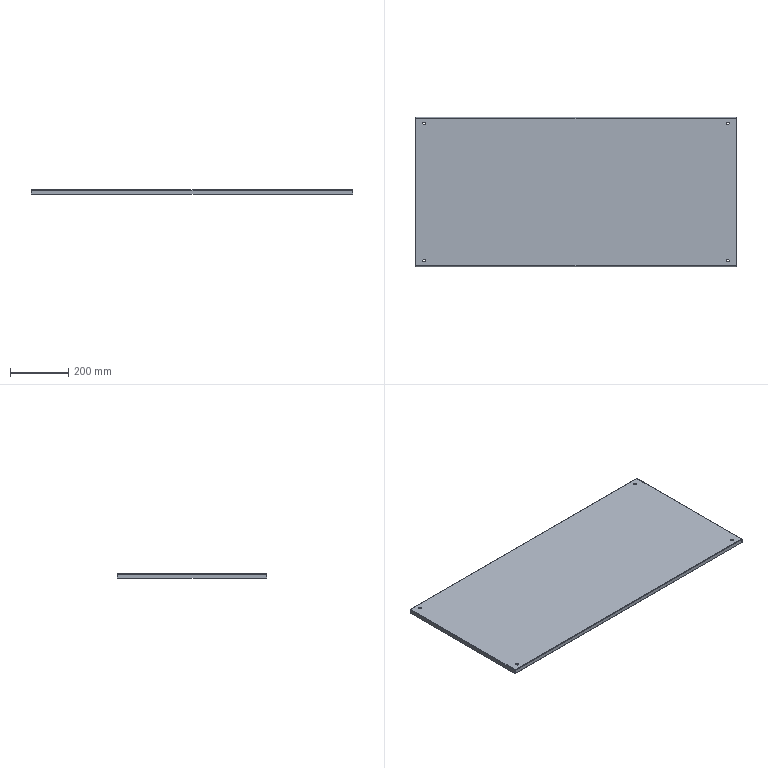Part | SolidWorks | features FlatPattern 1, ICE 1, SMBaseFlange 1, SMMiteredFlange 1, SheetMetal 1 | 1 solid | 46 faces | box 1100 x 510 x 15 mm | volume 902962 mm3 | plane 22 | cylinder 16 | spline 8 | commonest cylinder face diameters 9 x8 1.473 x4 4.473 x4